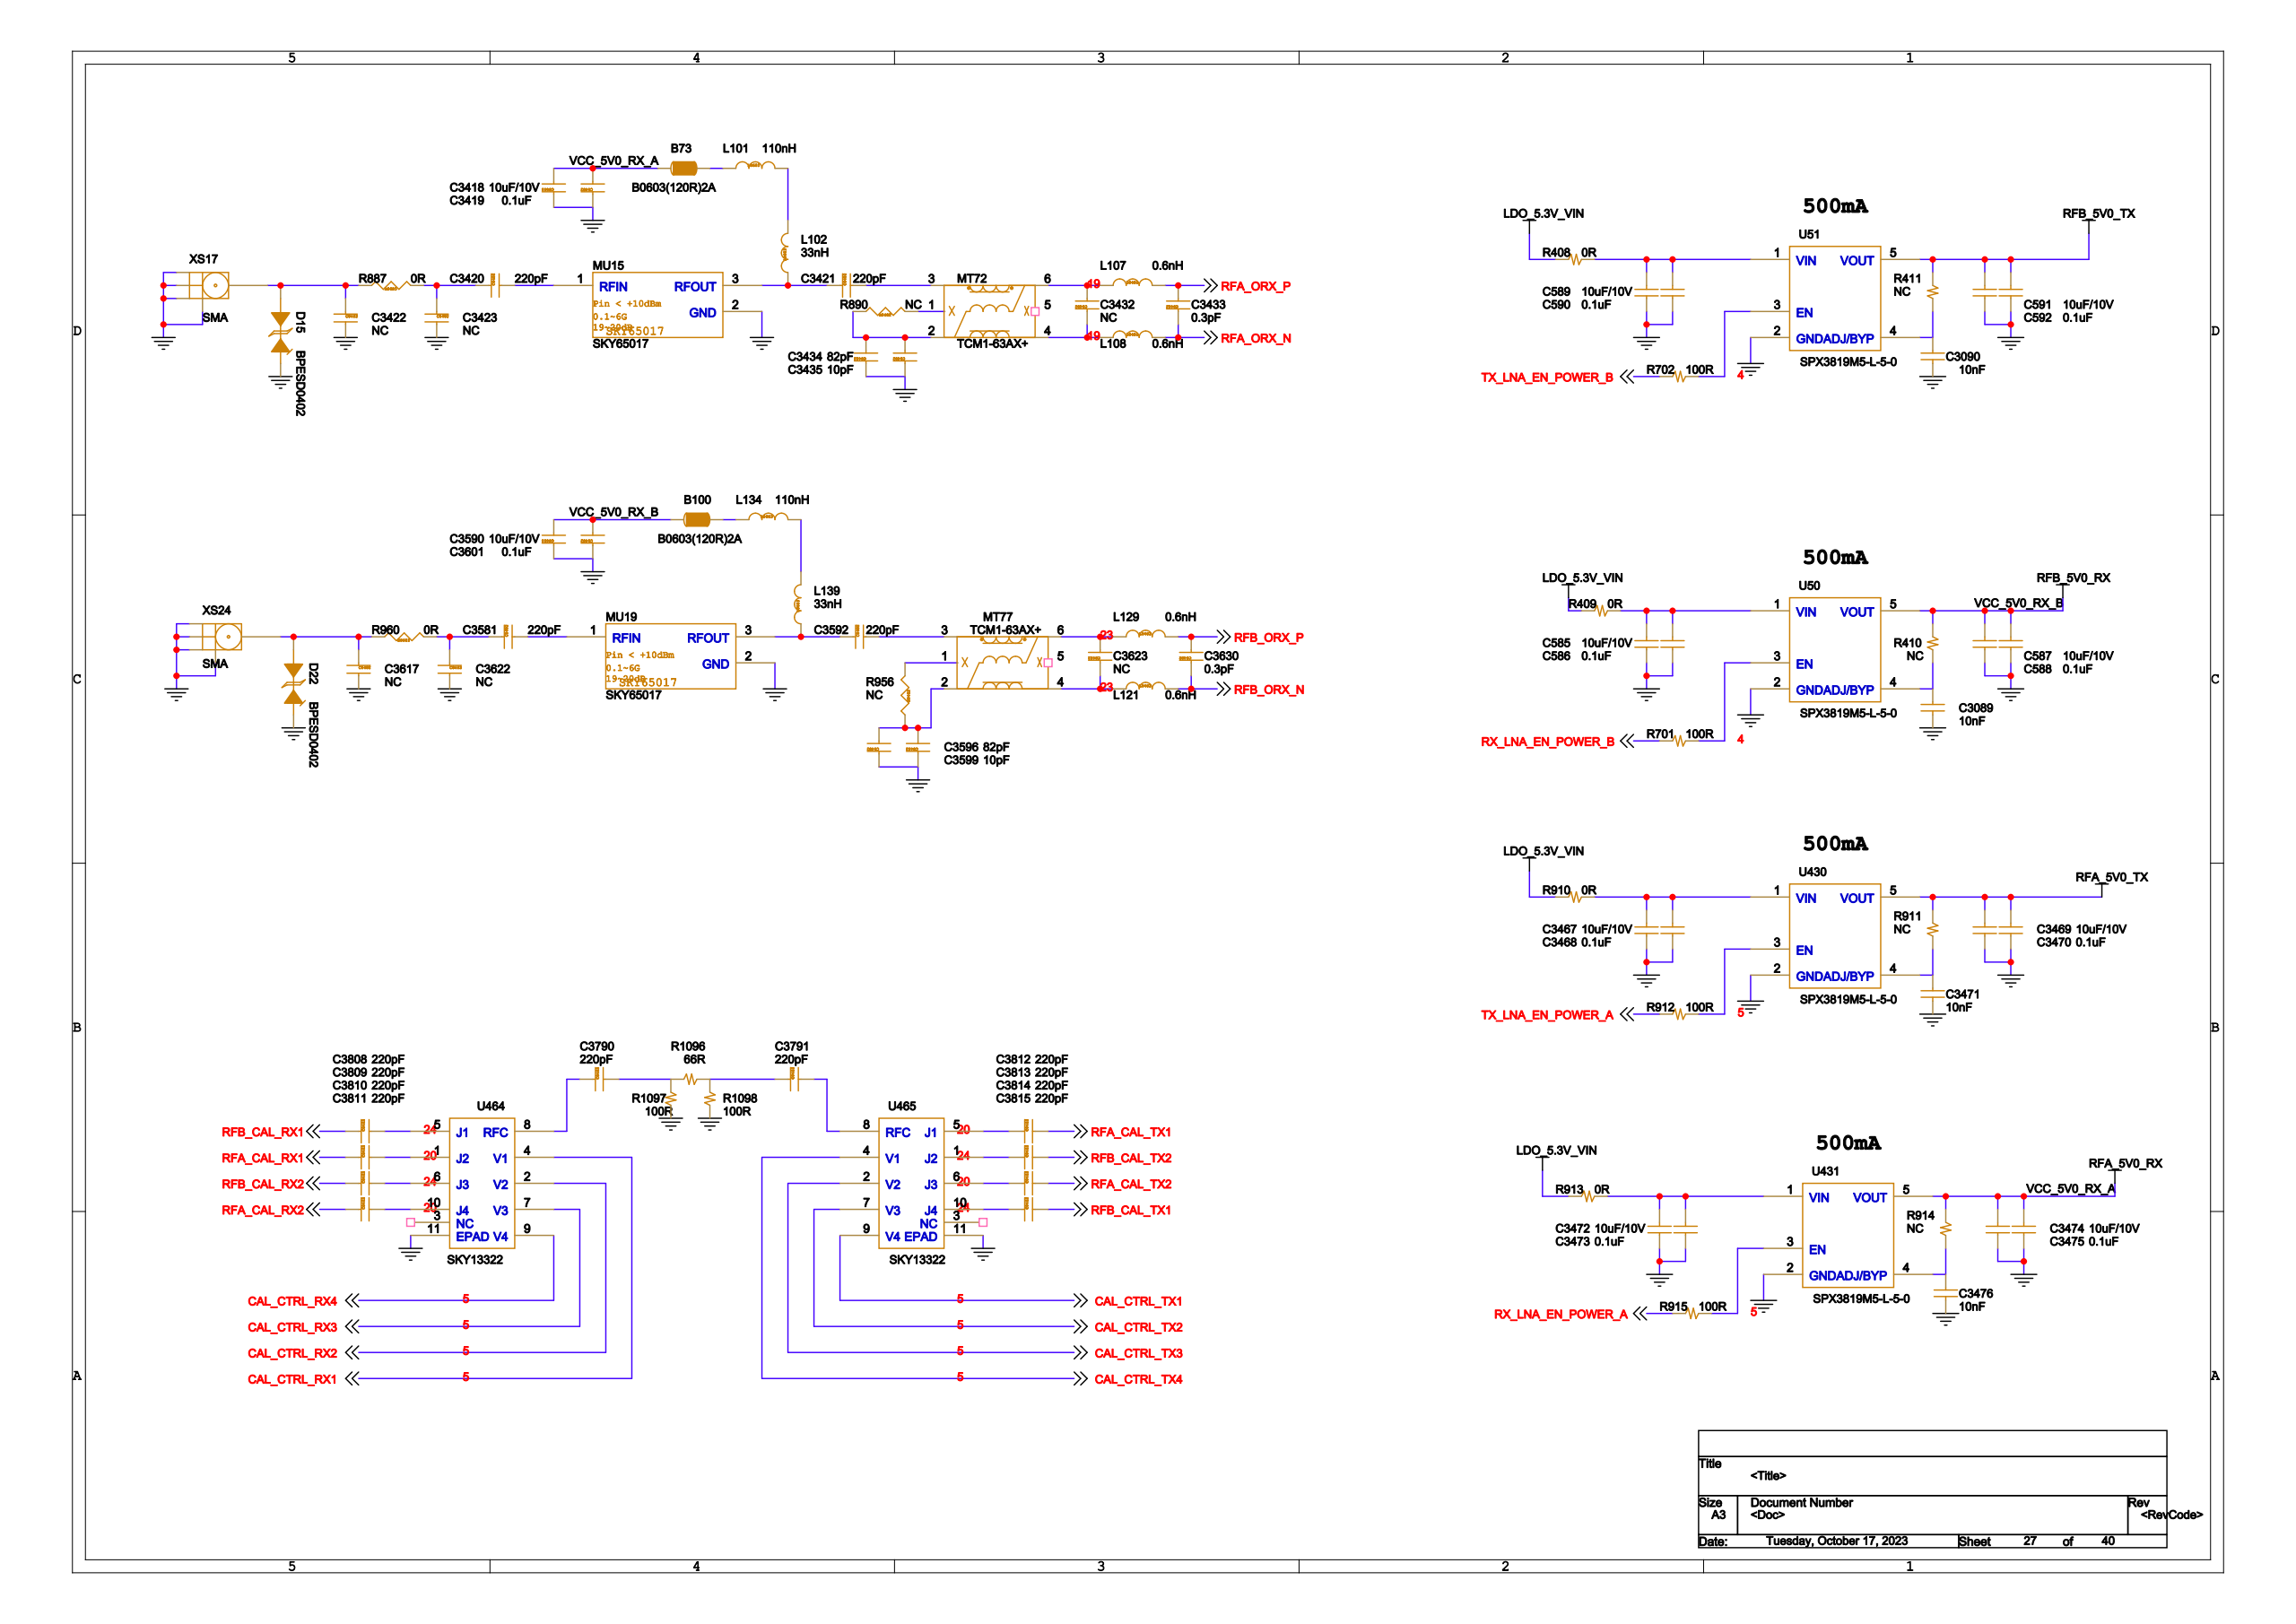Circuit board | Cadence Allegro | 1793 parts | 1223 nets | one sheet of the schematic
Parts on this sheet (reference | value | footprint):
B73 | B0603(120R)2A | B0603
B100 | B0603(120R)2A | B0603
C585 | 10uF/10V | C0402
C586 | 0.1uF | C0402
C587 | 10uF/10V | C0402
C588 | 0.1uF | C0402
C589 | 10uF/10V | C0402
C590 | 0.1uF | C0402
C591 | 10uF/10V | C0402
C592 | 0.1uF | C0402
C3089 | 10nF | C0402
C3090 | 10nF | C0402
C3418 | 10uF/10V | C0402
C3419 | 0.1uF | C0402
C3420 | 220pF | C0402
C3421 | 220pF | C0402
C3422 | NC | C0402
C3423 | NC | C0402
C3432 | NC | C0402
C3433 | 0.3pF | C0402
C3434 | 82pF | C0402
C3435 | 10pF | C0402
C3467 | 10uF/10V | C0402
C3468 | 0.1uF | C0402
C3469 | 10uF/10V | C0402
C3470 | 0.1uF | C0402
C3471 | 10nF | C0402
C3472 | 10uF/10V | C0402
C3473 | 0.1uF | C0402
C3474 | 10uF/10V | C0402
C3475 | 0.1uF | C0402
C3476 | 10nF | C0402
C3581 | 220pF | C0402
C3590 | 10uF/10V | C0402
C3592 | 220pF | C0402
C3596 | 82pF | C0402
C3599 | 10pF | C0402
C3601 | 0.1uF | C0402
C3617 | NC | C0402
C3622 | NC | C0402
C3623 | NC | C0402
C3630 | 0.3pF | C0402
C3790 | 220pF | C0402
C3791 | 220pF | C0402
C3808 | 220pF | C0402
C3809 | 220pF | C0402
C3810 | 220pF | C0402
C3811 | 220pF | C0402
C3812 | 220pF | C0402
C3813 | 220pF | C0402
C3814 | 220pF | C0402
C3815 | 220pF | C0402
D15 | BPESD0402 | C0402
D22 | BPESD0402 | C0402
L101 | 110nH | L0603
L102 | 33nH | L0603
L107 | 0.6nH | L0402
L108 | 0.6nH | L0402
L121 | 0.6nH | L0402
L129 | 0.6nH | L0402
L134 | 110nH | L0603
L139 | 33nH | L0603
MT72 | TCM1-63AX+ | TCM1-63AX
MT77 | TCM1-63AX+ | TCM1-63AX
MU15 | SKY65017 | SOT89_3
MU19 | SKY65017 | SOT89_3
R408 | 0R | R0402
R409 | 0R | R0402
R410 | NC | R0402
R411 | NC | R0402
R701 | 100R | R0402
R702 | 100R | R0402
R887 | 0R | R0603
R890 | NC | R0402
R910 | 0R | R0402
R911 | NC | R0402
R912 | 100R | R0402
R913 | 0R | R0402
R914 | NC | R0402
R915 | 100R | R0402
R956 | NC | R0402
R960 | 0R | R0603
R1096 | 66R | R0402
R1097 | 100R | R0402
R1098 | 100R | R0402
U50 | SPX3819M5-L-5-0 | SOT-23-5
U51 | SPX3819M5-L-5-0 | SOT-23-5
U430 | SPX3819M5-L-5-0 | SOT-23-5
U431 | SPX3819M5-L-5-0 | SOT-23-5
U464 | SKY13322 | LPD-10_L3_0-W2_0-P0_50-LS2_01
U465 | SKY13322 | LPD-10_L3_0-W2_0-P0_50-LS2_01
XS17 | SMA | SMA_5X5MM
XS24 | SMA | SMA_5X5MM
Nets of these parts (net: part-pin ...):
GND: C585-1 C586-1 C587-1 C588-1 C589-1 C590-1 C591-1 C592-1 C3089-2 C3090-2 C3418-1 C3419-1 C3422-2 C3423-2 C3434-1 C3435-1 C3467-1 C3468-1 C3469-1 C3470-1 C3471-2 C3472-1 C3473-1 C3474-1 C3475-1 C3476-2 C3590-1 C3596-1 C3599-1 C3601-1 C3617-2 C3622-2 D15-2 D22-2 MU15-2 MU19-2 R1097-1 R1098-1 U50-2 U51-2 U430-2 U431-2 U464-11 U465-11 XS17-2 XS17-3 XS17-4 XS17-5 XS24-2 XS24-3 XS24-4 XS24-5
N18610816: C3422-1 D15-1 R887-1 XS17-1
N18607344: C3617-1 D22-1 R960-1 XS24-1
LDO_5.3V_VIN: R408-1 R409-1 R910-1 R913-1
RFA_5V0_TX: C3469-2 C3470-2 R911-1 U430-5
RFA_5V0_RX: B73-1 C3418-2 C3419-2 C3474-2 C3475-2 R914-1 U431-5
RFB_5V0_TX: C591-2 C592-2 R411-1 U51-5
RFB_5V0_RX: B100-1 C587-2 C588-2 C3590-2 C3601-2 R410-1 U50-5
N18663377: C3790-2 R1096-1 R1097-2
N18663380: C3791-1 R1096-2 R1098-2
RFA_CAL_TX1: C3812-2
RFA_CAL_TX2: C3814-2
RFA_CAL_RX2: C3811-1
RFA_CAL_RX1: C3809-1
RFB_CAL_TX2: C3813-2
RFB_CAL_TX1: C3815-2
RFB_CAL_RX2: C3810-1
RFB_CAL_RX1: C3808-1
N18706161: C3808-2 U464-5
N18706158: C3809-2 U464-1
N18706155: C3810-2 U464-6
N18706152: C3811-2 U464-10
N18663562: C3790-1 U464-8
CAL_CTRL_RX1: U464-4
CAL_CTRL_RX2: U464-2
CAL_CTRL_RX3: U464-7
CAL_CTRL_RX4: U464-9
N18706276: C3812-1 U465-5
N18706288: C3813-1 U465-1
N18706298: C3814-1 U465-6
N18706308: C3815-1 U465-10
N18663569: C3791-2 U465-8
CAL_CTRL_TX4: U465-4
CAL_CTRL_TX3: U465-2
CAL_CTRL_TX2: U465-7
CAL_CTRL_TX1: U465-9
N18660794: C3467-2 C3468-2 R910-2 U430-1
N18660748: C3472-2 C3473-2 R913-2 U431-1
N18607509: C585-2 C586-2 R409-2 U50-1
N18607285: C589-2 C590-2 R408-2 U51-1
N18610830: C3420-2 MU15-1
N18610832: C3421-1 L102-2 MU15-3
N18607351: C3581-2 MU19-1
N18607352: C3592-1 L139-2 MU19-3
RFA_ORX_N: C3433-1 L108-2
RFA_ORX_P: C3433-2 L107-2
RFB_ORX_N: C3630-1 L121-2
RFB_ORX_P: C3630-2 L129-2
N18607338: B100-2 L134-2
N18610717: B73-2 L101-2
N18607525: C3089-1 R410-2 U50-4
N18607277: C3090-1 R411-2 U51-4
N18660929: C3471-1 R911-2 U430-4
N18660907: C3476-1 R914-2 U431-4
N18610824: C3420-1 C3423-1 R887-2
N18610922: C3432-1 L108-1 MT72-4
N18610850: C3432-2 L107-1 MT72-6
N18607348: C3581-1 C3622-1 R960-2
N18607390: C3623-1 L121-1 MT77-4
N18607386: C3623-2 L129-1 MT77-6
N18610836: C3421-2 MT72-3
N18607385: C3592-2 MT77-3
N18610914: C3434-2 C3435-2 MT72-2 R890-1
N18607392: C3596-2 C3599-2 MT77-2 R956-1
N18610719: L101-1 L102-1
N18607339: L134-1 L139-1
N18610916: MT72-1 R890-2
N18607389: MT77-1 R956-2
RX_LNA_EN_POWER_B: R701-1
N18607523: R701-2 U50-3
TX_LNA_EN_POWER_B: R702-1
N18607299: R702-2 U51-3
TX_LNA_EN_POWER_A: R912-1
N18660925: R912-2 U430-3
RX_LNA_EN_POWER_A: R915-1
N18660903: R915-2 U431-3